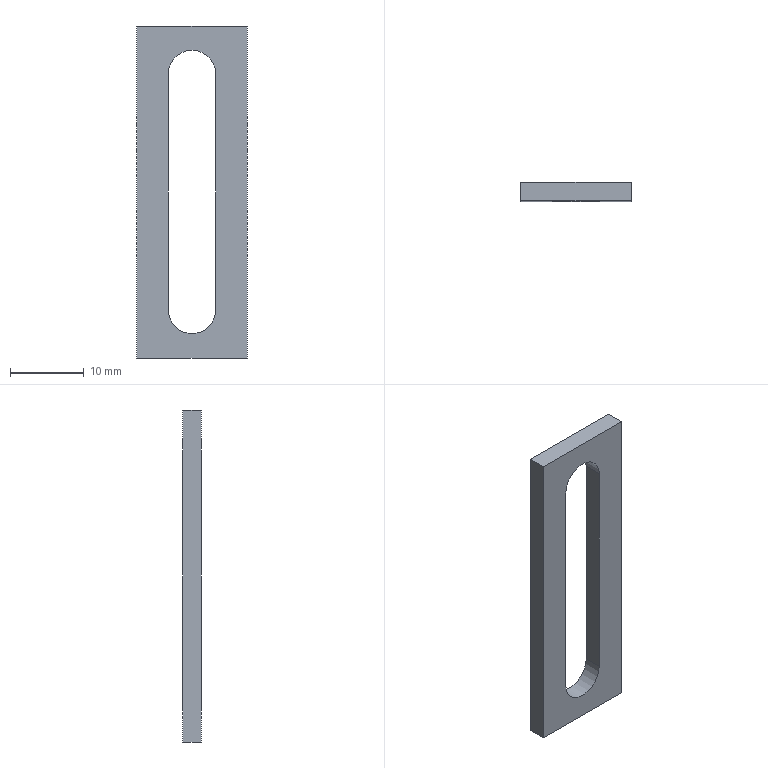Part | SolidWorks | features BaseBody 1 | 1 solid | 11 faces | box 15 x 2.5 x 45 mm | volume 1095 mm3 | plane 8 | cylinder 3 | commonest cylinder face diameters 6.4 x3
STEP:
#1=CARTESIAN_POINT('',(-3.2,2.5,-16.));
#2=VERTEX_POINT('',#1);
#3=CARTESIAN_POINT('',(3.2,2.5,-16.));
#4=VERTEX_POINT('',#3);
#5=CARTESIAN_POINT('',(0.,2.5,-16.));
#6=DIRECTION('',(0.,-1.,0.));
#7=DIRECTION('',(0.,0.,1.));
#8=AXIS2_PLACEMENT_3D('',#5,#6,#7);
#9=CIRCLE('',#8,3.2);
#10=EDGE_CURVE('',#2,#4,#9,.T.);
#11=ORIENTED_EDGE('',*,*,#10,.T.);
#12=CARTESIAN_POINT('',(3.2,2.5,16.));
#13=VERTEX_POINT('',#12);
#14=CARTESIAN_POINT('',(3.2,2.5,-16.));
#15=DIRECTION('',(0.,0.,1.));
#16=VECTOR('',#15,1000.);
#17=LINE('',#14,#16);
#18=EDGE_CURVE('',#4,#13,#17,.T.);
#19=ORIENTED_EDGE('',*,*,#18,.T.);
#20=CARTESIAN_POINT('',(0.,2.5,19.2));
#21=VERTEX_POINT('',#20);
#22=CARTESIAN_POINT('',(0.,2.5,16.));
#23=DIRECTION('',(0.,-1.,0.));
#24=DIRECTION('',(0.,0.,1.));
#25=AXIS2_PLACEMENT_3D('',#22,#23,#24);
#26=CIRCLE('',#25,3.2);
#27=EDGE_CURVE('',#13,#21,#26,.T.);
#28=ORIENTED_EDGE('',*,*,#27,.T.);
#29=CARTESIAN_POINT('',(-3.2,2.5,16.));
#30=VERTEX_POINT('',#29);
#31=CARTESIAN_POINT('',(0.,2.5,16.));
#32=DIRECTION('',(0.,-1.,0.));
#33=DIRECTION('',(0.,0.,1.));
#34=AXIS2_PLACEMENT_3D('',#31,#32,#33);
#35=CIRCLE('',#34,3.2);
#36=EDGE_CURVE('',#21,#30,#35,.T.);
#37=ORIENTED_EDGE('',*,*,#36,.T.);
#38=CARTESIAN_POINT('',(-3.2,2.5,-16.));
#39=DIRECTION('',(0.,0.,-1.));
#40=VECTOR('',#39,1000.);
#41=LINE('',#38,#40);
#42=EDGE_CURVE('',#30,#2,#41,.T.);
#43=ORIENTED_EDGE('',*,*,#42,.T.);
#44=EDGE_LOOP('',(#11,#19,#28,#37,#43));
#45=FACE_BOUND('',#44,.T.);
#46=CARTESIAN_POINT('',(7.5,2.5,22.5));
#47=VERTEX_POINT('',#46);
#48=CARTESIAN_POINT('',(7.5,2.5,-22.5));
#49=VERTEX_POINT('',#48);
#50=CARTESIAN_POINT('',(7.5,2.5,-22.5));
#51=DIRECTION('',(0.,0.,-1.));
#52=VECTOR('',#51,1000.);
#53=LINE('',#50,#52);
#54=EDGE_CURVE('',#47,#49,#53,.T.);
#55=ORIENTED_EDGE('',*,*,#54,.T.);
#56=CARTESIAN_POINT('',(-7.5,2.5,-22.5));
#57=VERTEX_POINT('',#56);
#58=CARTESIAN_POINT('',(-7.5,2.5,-22.5));
#59=DIRECTION('',(-1.,0.,0.));
#60=VECTOR('',#59,1000.);
#61=LINE('',#58,#60);
#62=EDGE_CURVE('',#49,#57,#61,.T.);
#63=ORIENTED_EDGE('',*,*,#62,.T.);
#64=CARTESIAN_POINT('',(-7.5,2.5,22.5));
#65=VERTEX_POINT('',#64);
#66=CARTESIAN_POINT('',(-7.5,2.5,-22.5));
#67=DIRECTION('',(0.,0.,1.));
#68=VECTOR('',#67,1000.);
#69=LINE('',#66,#68);
#70=EDGE_CURVE('',#57,#65,#69,.T.);
#71=ORIENTED_EDGE('',*,*,#70,.T.);
#72=CARTESIAN_POINT('',(-7.5,2.5,22.5));
#73=DIRECTION('',(1.,0.,0.));
#74=VECTOR('',#73,1000.);
#75=LINE('',#72,#74);
#76=EDGE_CURVE('',#65,#47,#75,.T.);
#77=ORIENTED_EDGE('',*,*,#76,.T.);
#78=EDGE_LOOP('',(#55,#63,#71,#77));
#79=FACE_OUTER_BOUND('',#78,.T.);
#80=CARTESIAN_POINT('',(0.,2.5,0.));
#81=DIRECTION('',(0.,1.,0.));
#82=DIRECTION('',(1.,0.,0.));
#83=AXIS2_PLACEMENT_3D('',#80,#81,#82);
#84=PLANE('',#83);
#85=ADVANCED_FACE('',(#45,#79),#84,.T.);
#86=ORIENTED_EDGE('',*,*,#54,.F.);
#87=CARTESIAN_POINT('',(7.5,0.,22.5));
#88=VERTEX_POINT('',#87);
#89=CARTESIAN_POINT('',(7.5,2.5,22.5));
#90=DIRECTION('',(0.,-1.,0.));
#91=VECTOR('',#90,1000.);
#92=LINE('',#89,#91);
#93=EDGE_CURVE('',#47,#88,#92,.T.);
#94=ORIENTED_EDGE('',*,*,#93,.T.);
#95=CARTESIAN_POINT('',(7.5,0.,-22.5));
#96=VERTEX_POINT('',#95);
#97=CARTESIAN_POINT('',(7.5,0.,0.));
#98=DIRECTION('',(0.,0.,-1.));
#99=VECTOR('',#98,1000.);
#100=LINE('',#97,#99);
#101=EDGE_CURVE('',#88,#96,#100,.T.);
#102=ORIENTED_EDGE('',*,*,#101,.T.);
#103=CARTESIAN_POINT('',(7.5,2.5,-22.5));
#104=DIRECTION('',(0.,1.,0.));
#105=VECTOR('',#104,1000.);
#106=LINE('',#103,#105);
#107=EDGE_CURVE('',#96,#49,#106,.T.);
#108=ORIENTED_EDGE('',*,*,#107,.T.);
#109=EDGE_LOOP('',(#86,#94,#102,#108));
#110=FACE_OUTER_BOUND('',#109,.T.);
#111=CARTESIAN_POINT('',(7.5,2.5,-22.5));
#112=DIRECTION('',(-1.,0.,0.));
#113=DIRECTION('',(0.,1.,0.));
#114=AXIS2_PLACEMENT_3D('',#111,#112,#113);
#115=PLANE('',#114);
#116=ADVANCED_FACE('',(#110),#115,.F.);
#117=ORIENTED_EDGE('',*,*,#62,.F.);
#118=ORIENTED_EDGE('',*,*,#107,.F.);
#119=CARTESIAN_POINT('',(-7.5,0.,-22.5));
#120=VERTEX_POINT('',#119);
#121=CARTESIAN_POINT('',(0.,0.,-22.5));
#122=DIRECTION('',(-1.,0.,0.));
#123=VECTOR('',#122,1000.);
#124=LINE('',#121,#123);
#125=EDGE_CURVE('',#96,#120,#124,.T.);
#126=ORIENTED_EDGE('',*,*,#125,.T.);
#127=CARTESIAN_POINT('',(-7.5,2.5,-22.5));
#128=DIRECTION('',(0.,1.,0.));
#129=VECTOR('',#128,1000.);
#130=LINE('',#127,#129);
#131=EDGE_CURVE('',#120,#57,#130,.T.);
#132=ORIENTED_EDGE('',*,*,#131,.T.);
#133=EDGE_LOOP('',(#117,#118,#126,#132));
#134=FACE_OUTER_BOUND('',#133,.T.);
#135=CARTESIAN_POINT('',(-7.5,2.5,-22.5));
#136=DIRECTION('',(0.,0.,1.));
#137=DIRECTION('',(1.,0.,0.));
#138=AXIS2_PLACEMENT_3D('',#135,#136,#137);
#139=PLANE('',#138);
#140=ADVANCED_FACE('',(#134),#139,.F.);
#141=ORIENTED_EDGE('',*,*,#70,.F.);
#142=ORIENTED_EDGE('',*,*,#131,.F.);
#143=CARTESIAN_POINT('',(-7.5,0.,22.5));
#144=VERTEX_POINT('',#143);
#145=CARTESIAN_POINT('',(-7.5,0.,0.));
#146=DIRECTION('',(0.,0.,1.));
#147=VECTOR('',#146,1000.);
#148=LINE('',#145,#147);
#149=EDGE_CURVE('',#120,#144,#148,.T.);
#150=ORIENTED_EDGE('',*,*,#149,.T.);
#151=CARTESIAN_POINT('',(-7.5,2.5,22.5));
#152=DIRECTION('',(0.,1.,0.));
#153=VECTOR('',#152,1000.);
#154=LINE('',#151,#153);
#155=EDGE_CURVE('',#144,#65,#154,.T.);
#156=ORIENTED_EDGE('',*,*,#155,.T.);
#157=EDGE_LOOP('',(#141,#142,#150,#156));
#158=FACE_OUTER_BOUND('',#157,.T.);
#159=CARTESIAN_POINT('',(-7.5,2.5,-22.5));
#160=DIRECTION('',(1.,0.,0.));
#161=DIRECTION('',(0.,0.,-1.));
#162=AXIS2_PLACEMENT_3D('',#159,#160,#161);
#163=PLANE('',#162);
#164=ADVANCED_FACE('',(#158),#163,.F.);
#165=ORIENTED_EDGE('',*,*,#76,.F.);
#166=ORIENTED_EDGE('',*,*,#155,.F.);
#167=CARTESIAN_POINT('',(0.,0.,22.5));
#168=DIRECTION('',(1.,0.,0.));
#169=VECTOR('',#168,1000.);
#170=LINE('',#167,#169);
#171=EDGE_CURVE('',#144,#88,#170,.T.);
#172=ORIENTED_EDGE('',*,*,#171,.T.);
#173=ORIENTED_EDGE('',*,*,#93,.F.);
#174=EDGE_LOOP('',(#165,#166,#172,#173));
#175=FACE_OUTER_BOUND('',#174,.T.);
#176=CARTESIAN_POINT('',(-7.5,2.5,22.5));
#177=DIRECTION('',(0.,0.,-1.));
#178=DIRECTION('',(0.,-1.,0.));
#179=AXIS2_PLACEMENT_3D('',#176,#177,#178);
#180=PLANE('',#179);
#181=ADVANCED_FACE('',(#175),#180,.F.);
#182=CARTESIAN_POINT('',(3.2,0.,-16.));
#183=VERTEX_POINT('',#182);
#184=CARTESIAN_POINT('',(3.2,0.,16.));
#185=VERTEX_POINT('',#184);
#186=CARTESIAN_POINT('',(3.2,0.,0.));
#187=DIRECTION('',(0.,0.,1.));
#188=VECTOR('',#187,1000.);
#189=LINE('',#186,#188);
#190=EDGE_CURVE('',#183,#185,#189,.T.);
#191=ORIENTED_EDGE('',*,*,#190,.T.);
#192=CARTESIAN_POINT('',(3.2,0.,16.));
#193=DIRECTION('',(0.,1.,0.));
#194=VECTOR('',#193,1000.);
#195=LINE('',#192,#194);
#196=EDGE_CURVE('',#185,#13,#195,.T.);
#197=ORIENTED_EDGE('',*,*,#196,.T.);
#198=ORIENTED_EDGE('',*,*,#18,.F.);
#199=CARTESIAN_POINT('',(3.2,0.,-16.));
#200=DIRECTION('',(0.,-1.,0.));
#201=VECTOR('',#200,1000.);
#202=LINE('',#199,#201);
#203=EDGE_CURVE('',#4,#183,#202,.T.);
#204=ORIENTED_EDGE('',*,*,#203,.T.);
#205=EDGE_LOOP('',(#191,#197,#198,#204));
#206=FACE_OUTER_BOUND('',#205,.T.);
#207=CARTESIAN_POINT('',(3.2,0.,-16.));
#208=DIRECTION('',(1.,0.,0.));
#209=DIRECTION('',(0.,0.,-1.));
#210=AXIS2_PLACEMENT_3D('',#207,#208,#209);
#211=PLANE('',#210);
#212=ADVANCED_FACE('',(#206),#211,.F.);
#213=CARTESIAN_POINT('',(0.,0.,19.2));
#214=VERTEX_POINT('',#213);
#215=CARTESIAN_POINT('',(0.,0.,19.2));
#216=DIRECTION('',(0.,1.,0.));
#217=VECTOR('',#216,1000.);
#218=LINE('',#215,#217);
#219=EDGE_CURVE('',#214,#21,#218,.T.);
#220=ORIENTED_EDGE('',*,*,#219,.F.);
#221=CARTESIAN_POINT('',(-3.2,0.,16.));
#222=VERTEX_POINT('',#221);
#223=CARTESIAN_POINT('',(0.,0.,16.));
#224=DIRECTION('',(0.,-1.,0.));
#225=DIRECTION('',(0.,0.,1.));
#226=AXIS2_PLACEMENT_3D('',#223,#224,#225);
#227=CIRCLE('',#226,3.2);
#228=EDGE_CURVE('',#214,#222,#227,.T.);
#229=ORIENTED_EDGE('',*,*,#228,.T.);
#230=CARTESIAN_POINT('',(-3.2,0.,16.));
#231=DIRECTION('',(0.,1.,0.));
#232=VECTOR('',#231,1000.);
#233=LINE('',#230,#232);
#234=EDGE_CURVE('',#222,#30,#233,.T.);
#235=ORIENTED_EDGE('',*,*,#234,.T.);
#236=ORIENTED_EDGE('',*,*,#36,.F.);
#237=EDGE_LOOP('',(#220,#229,#235,#236));
#238=FACE_OUTER_BOUND('',#237,.T.);
#239=CARTESIAN_POINT('',(0.,0.,16.));
#240=DIRECTION('',(0.,1.,0.));
#241=DIRECTION('',(0.,0.,1.));
#242=AXIS2_PLACEMENT_3D('',#239,#240,#241);
#243=CYLINDRICAL_SURFACE('',#242,3.2);
#244=ADVANCED_FACE('',(#238),#243,.F.);
#245=CARTESIAN_POINT('',(-3.2,0.,-16.));
#246=VERTEX_POINT('',#245);
#247=CARTESIAN_POINT('',(-3.2,0.,0.));
#248=DIRECTION('',(0.,0.,-1.));
#249=VECTOR('',#248,1000.);
#250=LINE('',#247,#249);
#251=EDGE_CURVE('',#222,#246,#250,.T.);
#252=ORIENTED_EDGE('',*,*,#251,.T.);
#253=CARTESIAN_POINT('',(-3.2,0.,-16.));
#254=DIRECTION('',(0.,1.,0.));
#255=VECTOR('',#254,1000.);
#256=LINE('',#253,#255);
#257=EDGE_CURVE('',#246,#2,#256,.T.);
#258=ORIENTED_EDGE('',*,*,#257,.T.);
#259=ORIENTED_EDGE('',*,*,#42,.F.);
#260=ORIENTED_EDGE('',*,*,#234,.F.);
#261=EDGE_LOOP('',(#252,#258,#259,#260));
#262=FACE_OUTER_BOUND('',#261,.T.);
#263=CARTESIAN_POINT('',(-3.2,0.,-16.));
#264=DIRECTION('',(-1.,0.,0.));
#265=DIRECTION('',(0.,1.,0.));
#266=AXIS2_PLACEMENT_3D('',#263,#264,#265);
#267=PLANE('',#266);
#268=ADVANCED_FACE('',(#262),#267,.F.);
#269=CARTESIAN_POINT('',(0.,0.,-16.));
#270=DIRECTION('',(0.,-1.,0.));
#271=DIRECTION('',(0.,0.,1.));
#272=AXIS2_PLACEMENT_3D('',#269,#270,#271);
#273=CIRCLE('',#272,3.2);
#274=EDGE_CURVE('',#246,#183,#273,.T.);
#275=ORIENTED_EDGE('',*,*,#274,.T.);
#276=ORIENTED_EDGE('',*,*,#203,.F.);
#277=ORIENTED_EDGE('',*,*,#10,.F.);
#278=ORIENTED_EDGE('',*,*,#257,.F.);
#279=EDGE_LOOP('',(#275,#276,#277,#278));
#280=FACE_OUTER_BOUND('',#279,.T.);
#281=CARTESIAN_POINT('',(0.,0.,-16.));
#282=DIRECTION('',(0.,1.,0.));
#283=DIRECTION('',(0.,0.,1.));
#284=AXIS2_PLACEMENT_3D('',#281,#282,#283);
#285=CYLINDRICAL_SURFACE('',#284,3.2);
#286=ADVANCED_FACE('',(#280),#285,.F.);
#287=ORIENTED_EDGE('',*,*,#251,.F.);
#288=ORIENTED_EDGE('',*,*,#228,.F.);
#289=CARTESIAN_POINT('',(0.,0.,16.));
#290=DIRECTION('',(0.,-1.,0.));
#291=DIRECTION('',(0.,0.,1.));
#292=AXIS2_PLACEMENT_3D('',#289,#290,#291);
#293=CIRCLE('',#292,3.2);
#294=EDGE_CURVE('',#185,#214,#293,.T.);
#295=ORIENTED_EDGE('',*,*,#294,.F.);
#296=ORIENTED_EDGE('',*,*,#190,.F.);
#297=ORIENTED_EDGE('',*,*,#274,.F.);
#298=EDGE_LOOP('',(#287,#288,#295,#296,#297));
#299=FACE_BOUND('',#298,.T.);
#300=ORIENTED_EDGE('',*,*,#149,.F.);
#301=ORIENTED_EDGE('',*,*,#125,.F.);
#302=ORIENTED_EDGE('',*,*,#101,.F.);
#303=ORIENTED_EDGE('',*,*,#171,.F.);
#304=EDGE_LOOP('',(#300,#301,#302,#303));
#305=FACE_OUTER_BOUND('',#304,.T.);
#306=CARTESIAN_POINT('',(0.,0.,0.));
#307=DIRECTION('',(0.,1.,0.));
#308=DIRECTION('',(1.,0.,0.));
#309=AXIS2_PLACEMENT_3D('',#306,#307,#308);
#310=PLANE('',#309);
#311=ADVANCED_FACE('',(#299,#305),#310,.F.);
#312=ORIENTED_EDGE('',*,*,#294,.T.);
#313=ORIENTED_EDGE('',*,*,#219,.T.);
#314=ORIENTED_EDGE('',*,*,#27,.F.);
#315=ORIENTED_EDGE('',*,*,#196,.F.);
#316=EDGE_LOOP('',(#312,#313,#314,#315));
#317=FACE_OUTER_BOUND('',#316,.T.);
#318=CARTESIAN_POINT('',(0.,0.,16.));
#319=DIRECTION('',(0.,1.,0.));
#320=DIRECTION('',(0.,0.,1.));
#321=AXIS2_PLACEMENT_3D('',#318,#319,#320);
#322=CYLINDRICAL_SURFACE('',#321,3.2);
#323=ADVANCED_FACE('',(#317),#322,.F.);
#324=CLOSED_SHELL('',(#85,#116,#140,#164,#181,#212,#244,#268,#286,#311,#323));
#325=MANIFOLD_SOLID_BREP('',#324);
#326=CARTESIAN_POINT('',(0.,0.,0.));
#327=DIRECTION('',(0.,0.,1.));
#328=DIRECTION('',(1.,0.,0.));
#329=AXIS2_PLACEMENT_3D('',#326,#327,#328);
#330=(LENGTH_UNIT()NAMED_UNIT(*)SI_UNIT(.MILLI.,.METRE.));
#331=UNCERTAINTY_MEASURE_WITH_UNIT(LENGTH_MEASURE(0.00001),#330,'','');
#332=(NAMED_UNIT(*)PLANE_ANGLE_UNIT()SI_UNIT($,.RADIAN.));
#333=(NAMED_UNIT(*)SI_UNIT($,.STERADIAN.)SOLID_ANGLE_UNIT());
#334=(GEOMETRIC_REPRESENTATION_CONTEXT(3)GLOBAL_UNCERTAINTY_ASSIGNED_CONTEXT((#331))GLOBAL_UNIT_ASSIGNED_CONTEXT((#330,#332,#333))REPRESENTATION_CONTEXT('',''));
#335=ADVANCED_BREP_SHAPE_REPRESENTATION('',(#325,#329),#334);